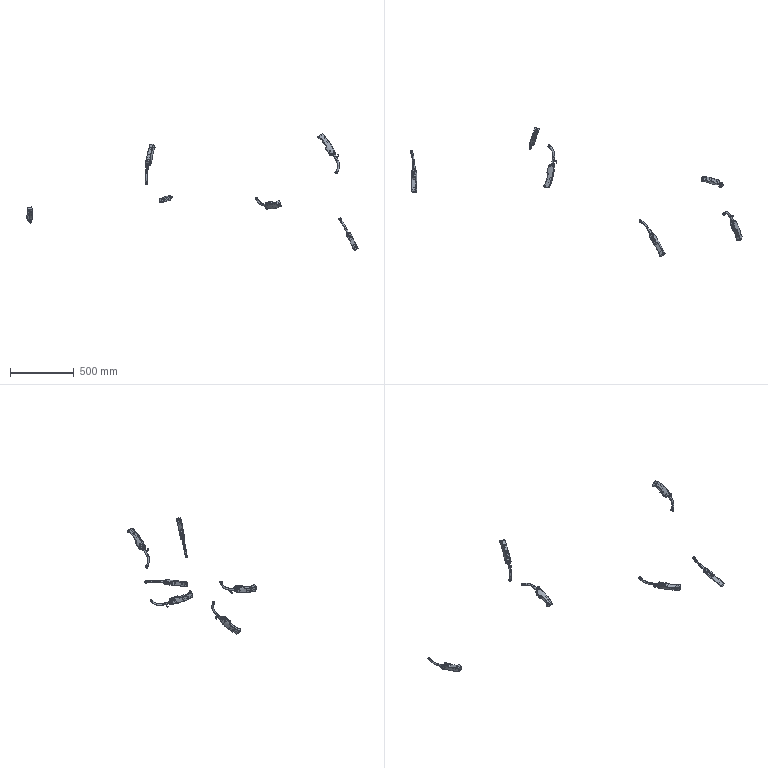Part | STEP file | TOCHA-1-SOLID3 | 6 solids | 1674 faces | box 2607 x 1013 x 916.163 mm | volume 1110873 mm3 | plane 720 | cylinder 546 | spline 204 | torus 96 | cone 96 | other 12 | commonest cylinder face diameters 4.75 x36 15.748 x36 25.4 x30 4.318 x24 14.326 x24 19.05 x24